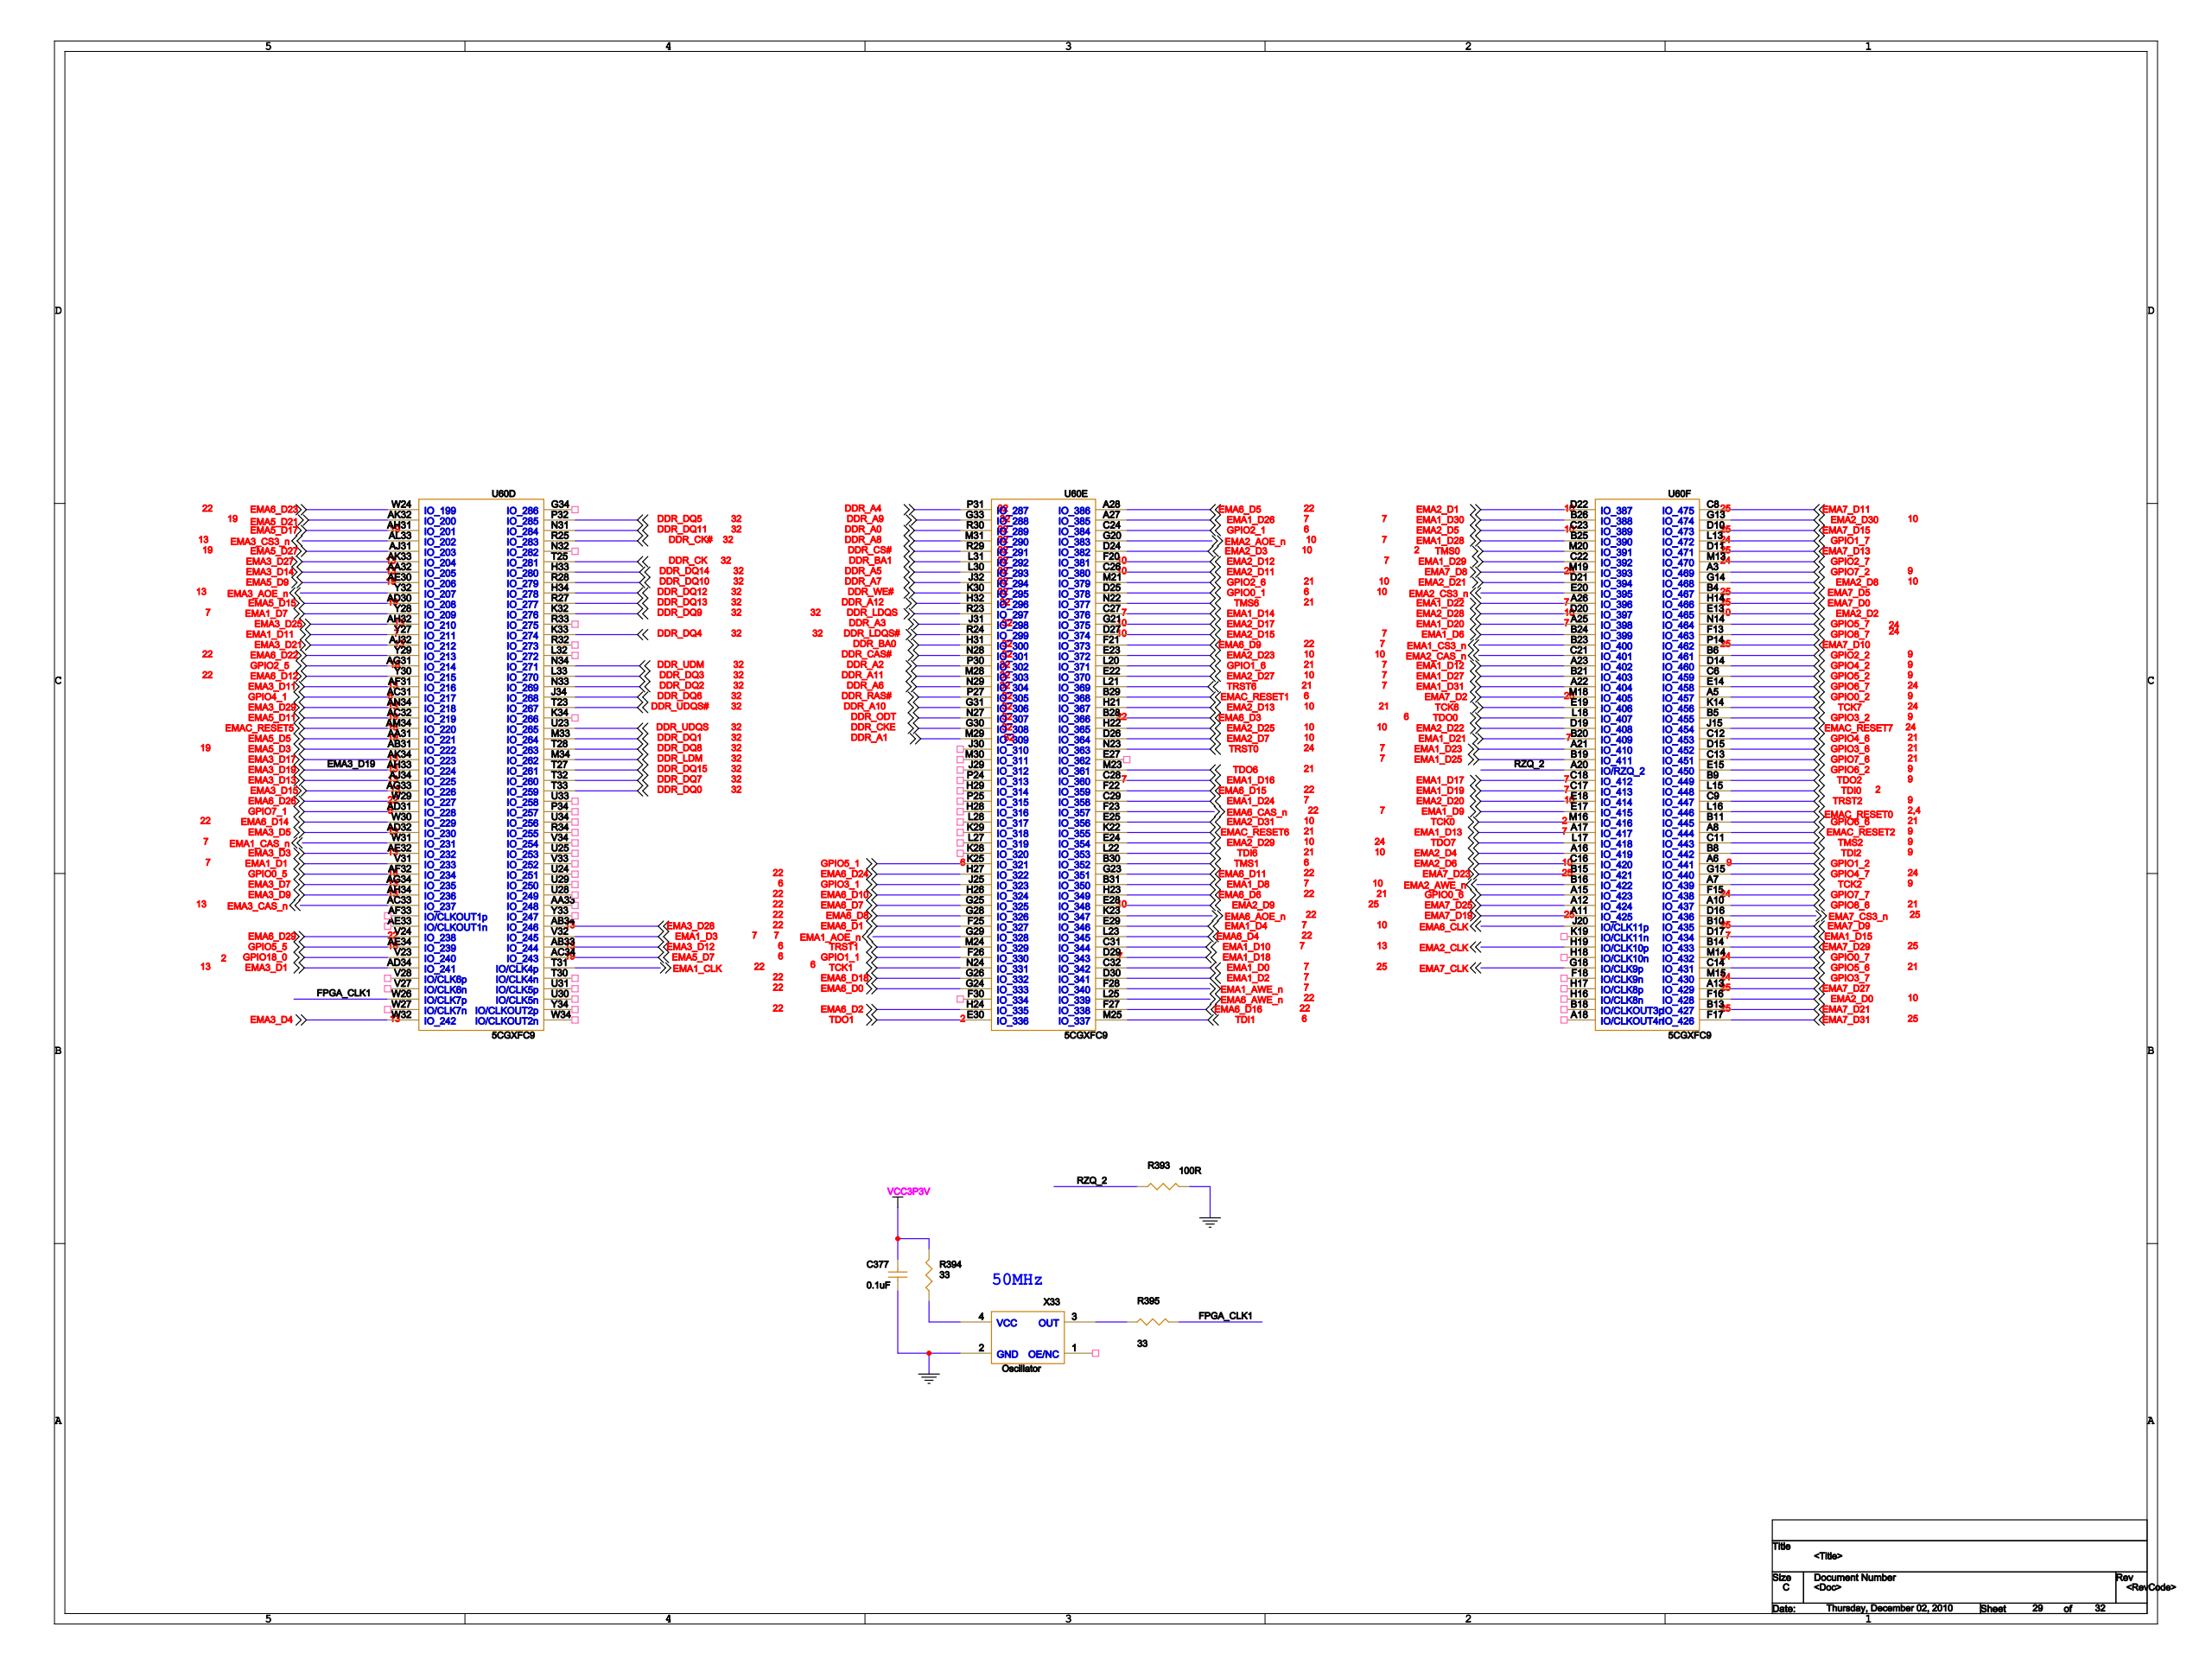Circuit board | Cadence Allegro | 1001 parts | 1318 nets | one sheet of the schematic
Parts on this sheet (reference | value | footprint):
C26 | 0.1uF | C0402
C27 | 0.1uF | C0402
C29 | 0.1uF | C0402
C377 | 0.1uF | 0603
R393 | 100R | 0603
R394 | 33 | 0603
R395 | 33 | 0603
U23 | MT48LC32M16 | TSOP54
U28 | SoC_HTC_01 | L529_XIN
U29 | MT48LC32M16 | TSOP54
U33 | MT48LC16M16 | TSOP54
U34 | SoC_HTC_01 | L529_XIN
U60 | 5CGXFC9 | FBGA1152
X33 | Oscillator | OSC_5_7
Nets of these parts (net: part-pin ...):
EMA5_D5: U60-AA31
EMA3_D14: U60-AA32
EMA5_D3: U60-AB31
EMA3_D12: U60-AB33
EMA3_D28: U60-AB34
GPIO4_1: U60-AC31
EMA5_D11: U60-AC32
EMA5_D7: U60-AC34
EMA5_D15: U60-AD30
GPIO7_1: U60-AD31
EMA3_D5: U60-AD32
EMA3_D1: U60-AD34
EMA5_D9: U60-AE30
EMA3_D3: U60-AE32
GPIO5_5: U34-E15 U60-AE34
EMA3_D11: U60-AF31
GPIO0_5: U34-D14 U60-AF32
GPIO2_5: U34-E14 U60-AG31
EMA3_D15: U60-AG33
EMA3_D7: U60-AG34
EMA5_D17: U60-AH31
EMA3_D25: U60-AH32
EMA3_D19: U60-AH33
EMA3_D9: U60-AH34
EMA5_D27: U60-AJ31
EMA3_D21: U60-AJ32
EMA3_D13: U60-AJ34
EMA5_D21: U60-AK32
EMA3_D27: U60-AK33
EMA3_D17: U60-AK34
EMAC_RESET5: U60-AM34
EMA3_D29: U60-AN34
DDR_DQ14: U60-H33
DDR_DQ12: U60-H34
DDR_DQ6: U60-J34
DDR_DQ9: U60-K32
DDR_DQ4: U60-K33
DDR_DQ3: U60-L33
DDR_DQ1: U60-M33
DDR_LDM: U60-M34
DDR_DQ11: U60-N31
DDR_DQ2: U60-N33
DDR_UDM: U60-N34
DDR_DQ5: U60-P32
DDR_CK#: U60-R25
DDR_DQ13: U60-R27
DDR_DQ10: U60-R28
DDR_UDQS#: U60-T23
DDR_CK: U60-T25
DDR_DQ15: U60-T27
DDR_DQ8: U60-T28
DDR_DQ7: U60-T32
DDR_DQ0: U60-T33
DDR_UDQS: U60-U23
GPIO18_0: U60-V23
EMA6_D29: U60-V24
EMA1_D1: U60-V31
EMA1_D3: U60-V32
EMA6_D23: U60-W24
EMA6_D26: U60-W29
EMA6_D14: U60-W30
EMA3_D4: U60-W32
EMA1_D11: U60-Y27
EMA1_D7: U60-Y28
EMA6_D22: U60-Y29
EMA6_D12: U60-Y30
EMA1_CLK: U60-T31
FPGA_CLK1: R395-2 U60-W26
EMA1_D26: U60-A27
EMA6_D5: U60-A28
EMA6_D3: U60-B28
EMAC_RESET1: U60-B29
TMS1: U60-B30
EMA1_D8: U60-B31
GPIO2_1: U60-C24
EMA2_D11: U60-C26
EMA1_D14: U60-C27
EMA1_D16: U60-C28
EMA1_D24: U60-C29
EMA1_D10: U60-C31
EMA1_D0: U60-C32
EMA2_D3: U60-D24
GPIO0_1: U60-D25
EMA2_D7: U60-D26
EMA2_D15: U60-D27
EMA1_D18: U60-D29
EMA1_D2: U60-D30
EMA2_D27: U60-E22
EMA2_D23: U60-E23
EMA2_D29: U60-E24
EMA2_D31: U60-E25
EMA2_D9: U60-E28
EMA1_D4: U60-E29
TDO1: U60-E30
EMA2_D12: U60-F20
EMA6_D9: U60-F21
EMA6_D15: U60-F22
EMA6_D1: U60-F25
GPIO1_1: U60-F26
EMA6_D16: U60-F27
EMA2_D17: U60-G21
EMA6_D11: U60-G23
EMA6_D0: U60-G24
EMA6_D7: U60-G25
EMA6_D18: U60-G26
EMA6_D8: U60-G28
DDR_CKE: U60-G30
DDR_A10: U60-G31
DDR_A9: U60-G33
EMA2_D13: U60-H21
EMA2_D25: U60-H22
EMA6_D6: U60-H23
EMA6_D2: U60-H24
EMA6_D10: U60-H26
EMA6_D24: U60-H27
DDR_BA0: U60-H31
DDR_A12: U60-H32
GPIO3_1: U60-J25
DDR_A3: U60-J31
DDR_A7: U60-J32
EMAC_RESET6: U60-K22
GPIO5_1: U60-K25
DDR_WE#: U60-K30
GPIO1_6: U60-L20
TRST6: U60-L21
TDI6: U60-L22
EMA6_D4: U60-L23
DDR_A5: U60-L30
DDR_BA1: U60-L31
GPIO2_6: U60-M21
TDO6: U60-M23
TRST1: U60-M24
TDI1: U60-M25
DDR_A11: U60-M28
DDR_A1: U60-M29
DDR_A8: U60-M31
TMS6: U60-N22
TRST0: U60-N23
TCK1: U60-N24
DDR_ODT: U60-N27
DDR_CAS#: U60-N28
DDR_A6: U60-N29
DDR_RAS#: U60-P27
DDR_A2: U60-P30
DDR_A4: U60-P31
DDR_LDQS: U60-R23
DDR_LDQS#: U60-R24
DDR_CS#: U60-R29
DDR_A0: U60-R30
GPIO8_6: U60-A10
EMA7_D19: U60-A11
EMA7_D25: U60-A12
EMA7_D27: U60-A13
GPIO0_6: U60-A15
EMA2_D4: U60-A16
EMA1_D13: U60-A17
EMA1_D23: U60-A21
EMA1_D31: U60-A22
EMA1_D12: U60-A23
EMA1_D20: U60-A25
EMA1_D22: U60-A26
GPIO7_2: U60-A3
GPIO0_2: U60-A5
GPIO1_2: U60-A6
TCK2: U60-A7
EMAC_RESET2: U60-A8
EMA7_D9: U60-B10
GPIO6_6: U60-B11
EMA7_D21: U60-B13
EMA7_D29: U60-B14
EMA7_D23: U60-B15
EMA1_D25: U60-B19
EMA1_D21: U60-B20
EMA1_D27: U60-B21
EMA1_D6: U60-B24
EMA1_D28: U60-B25
EMA1_D30: U60-B26
EMA7_D5: U60-B4
GPIO3_2: U60-B5
GPIO2_2: U60-B6
TDI2: U60-B8
TDO2: U60-B9
TMS2: U60-C11
GPIO4_6: U60-C12
GPIO7_6: U60-C13
GPIO5_6: U60-C14
EMA2_D6: U60-C16
EMA1_D19: U60-C17
EMA1_D17: U60-C18
EMA1_D29: U60-C22
EMA2_D5: U60-C23
GPIO5_2: U60-C6
EMA7_D11: U60-C8
TRST2: U60-C9
EMA7_D15: U60-D10
EMA7_D13: U60-D11
GPIO4_2: U60-D14
GPIO3_6: U60-D15
EMA1_D15: U60-D17
EMA2_D22: U60-D19
EMA2_D28: U60-D20
EMA2_D21: U60-D21
EMA2_D1: U60-D22
EMA2_D2: U60-E13
GPIO6_7: U60-E14
GPIO6_2: U60-E15
EMA1_D9: U60-E17
EMA2_D20: U60-E18
TCK6: U60-E19
GPIO8_7: U60-F13
GPIO7_7: U60-F15
EMA2_D0: U60-F16
EMA7_D31: U60-F17
EMA2_D30: U60-G13
EMA2_D8: U60-G14
GPIO4_7: U60-G15
EMA7_D0: U60-H14
EMAC_RESET7: U60-J15
TCK7: U60-K14
GPIO1_7: U60-L13
TDI0: U60-L15
EMAC_RESET0: U60-L16
TDO7: U60-L17
TDO0: U60-L18
GPIO2_7: U60-M13
GPIO0_7: U60-M14
GPIO3_7: U60-M15
TCK0: U60-M16
EMA7_D2: U60-M18
EMA7_D8: U60-M19
TMS0: U60-M20
GPIO5_7: U60-N14
EMA7_D10: U60-P14
EMA2_CLK: U60-H19
EMA6_CLK: U60-J20
EMA7_CLK: U60-G18
RZQ_2: R393-1 U60-A20
GND: C26-2 C27-2 C29-2 C377-2 R393-2 X33-2 U23-6 U28-A6 U28-A7 U28-B6 U28-B15 U28-B16 U28-B19 U28-C11 U28-C13 U28-C22 U28-E18 U28-F15 U28-F22 U28-G14 U28-H16 U28-H22 U28-H23 U28-K14 U28-L16 U28-L18 U28-N23 U29-6 U33-6 U34-A6 U34-A7 U34-B6 U34-B15 U34-B16 U34-B19 U34-C11 U34-C13 U34-C22 U34-E18 U34-F15 U34-F22 U34-G14 U34-H16 U34-H22 U34-H23 U34-K14 U34-L16 U34-L18 U34-N23
VCC3P3V: C377-1 R394-2 U23-1 U23-3 U23-9 U28-B5 U28-D19 U28-H14 U28-H18 U28-J20 U28-L15 U28-L17 U29-1 U29-3 U29-9 U33-1 U33-3 U33-9 U34-B5 U34-D19 U34-H14 U34-H18 U34-J20 U34-L15 U34-L17
3V3_MEM: C26-1 C27-1 U28-D17 U28-G23 U28-M20 U34-D17 U34-G23 U34-M20
1V2_MEM: C29-1 U28-A8 U28-A15 U28-C12 U28-D21 U28-E13 U28-G18 U28-H21 U28-M18 U34-A8 U34-A15 U34-C12 U34-D21 U34-E13 U34-G18 U34-H21 U34-M18
N17368118: R394-1 X33-4
N17368136: R395-1 X33-3